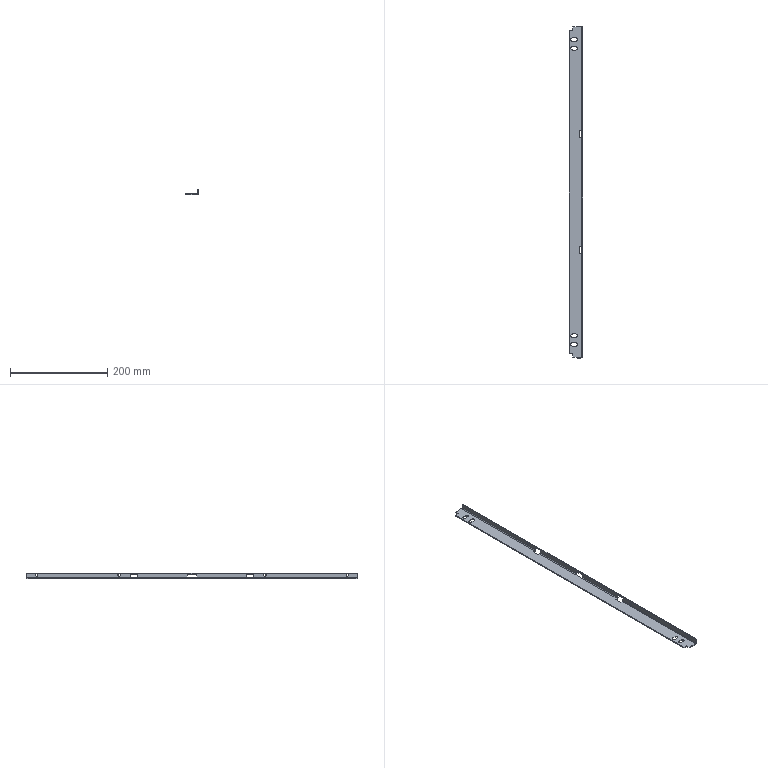Part | STEP file | Gasket strip horizontal (flat door) modified | 1 solid | 81 faces | box 28.5 x 684 x 12 mm | volume 48634 mm3 | plane 53 | cylinder 28 | commonest cylinder face diameters 7 x16 5.3 x8 3 x4